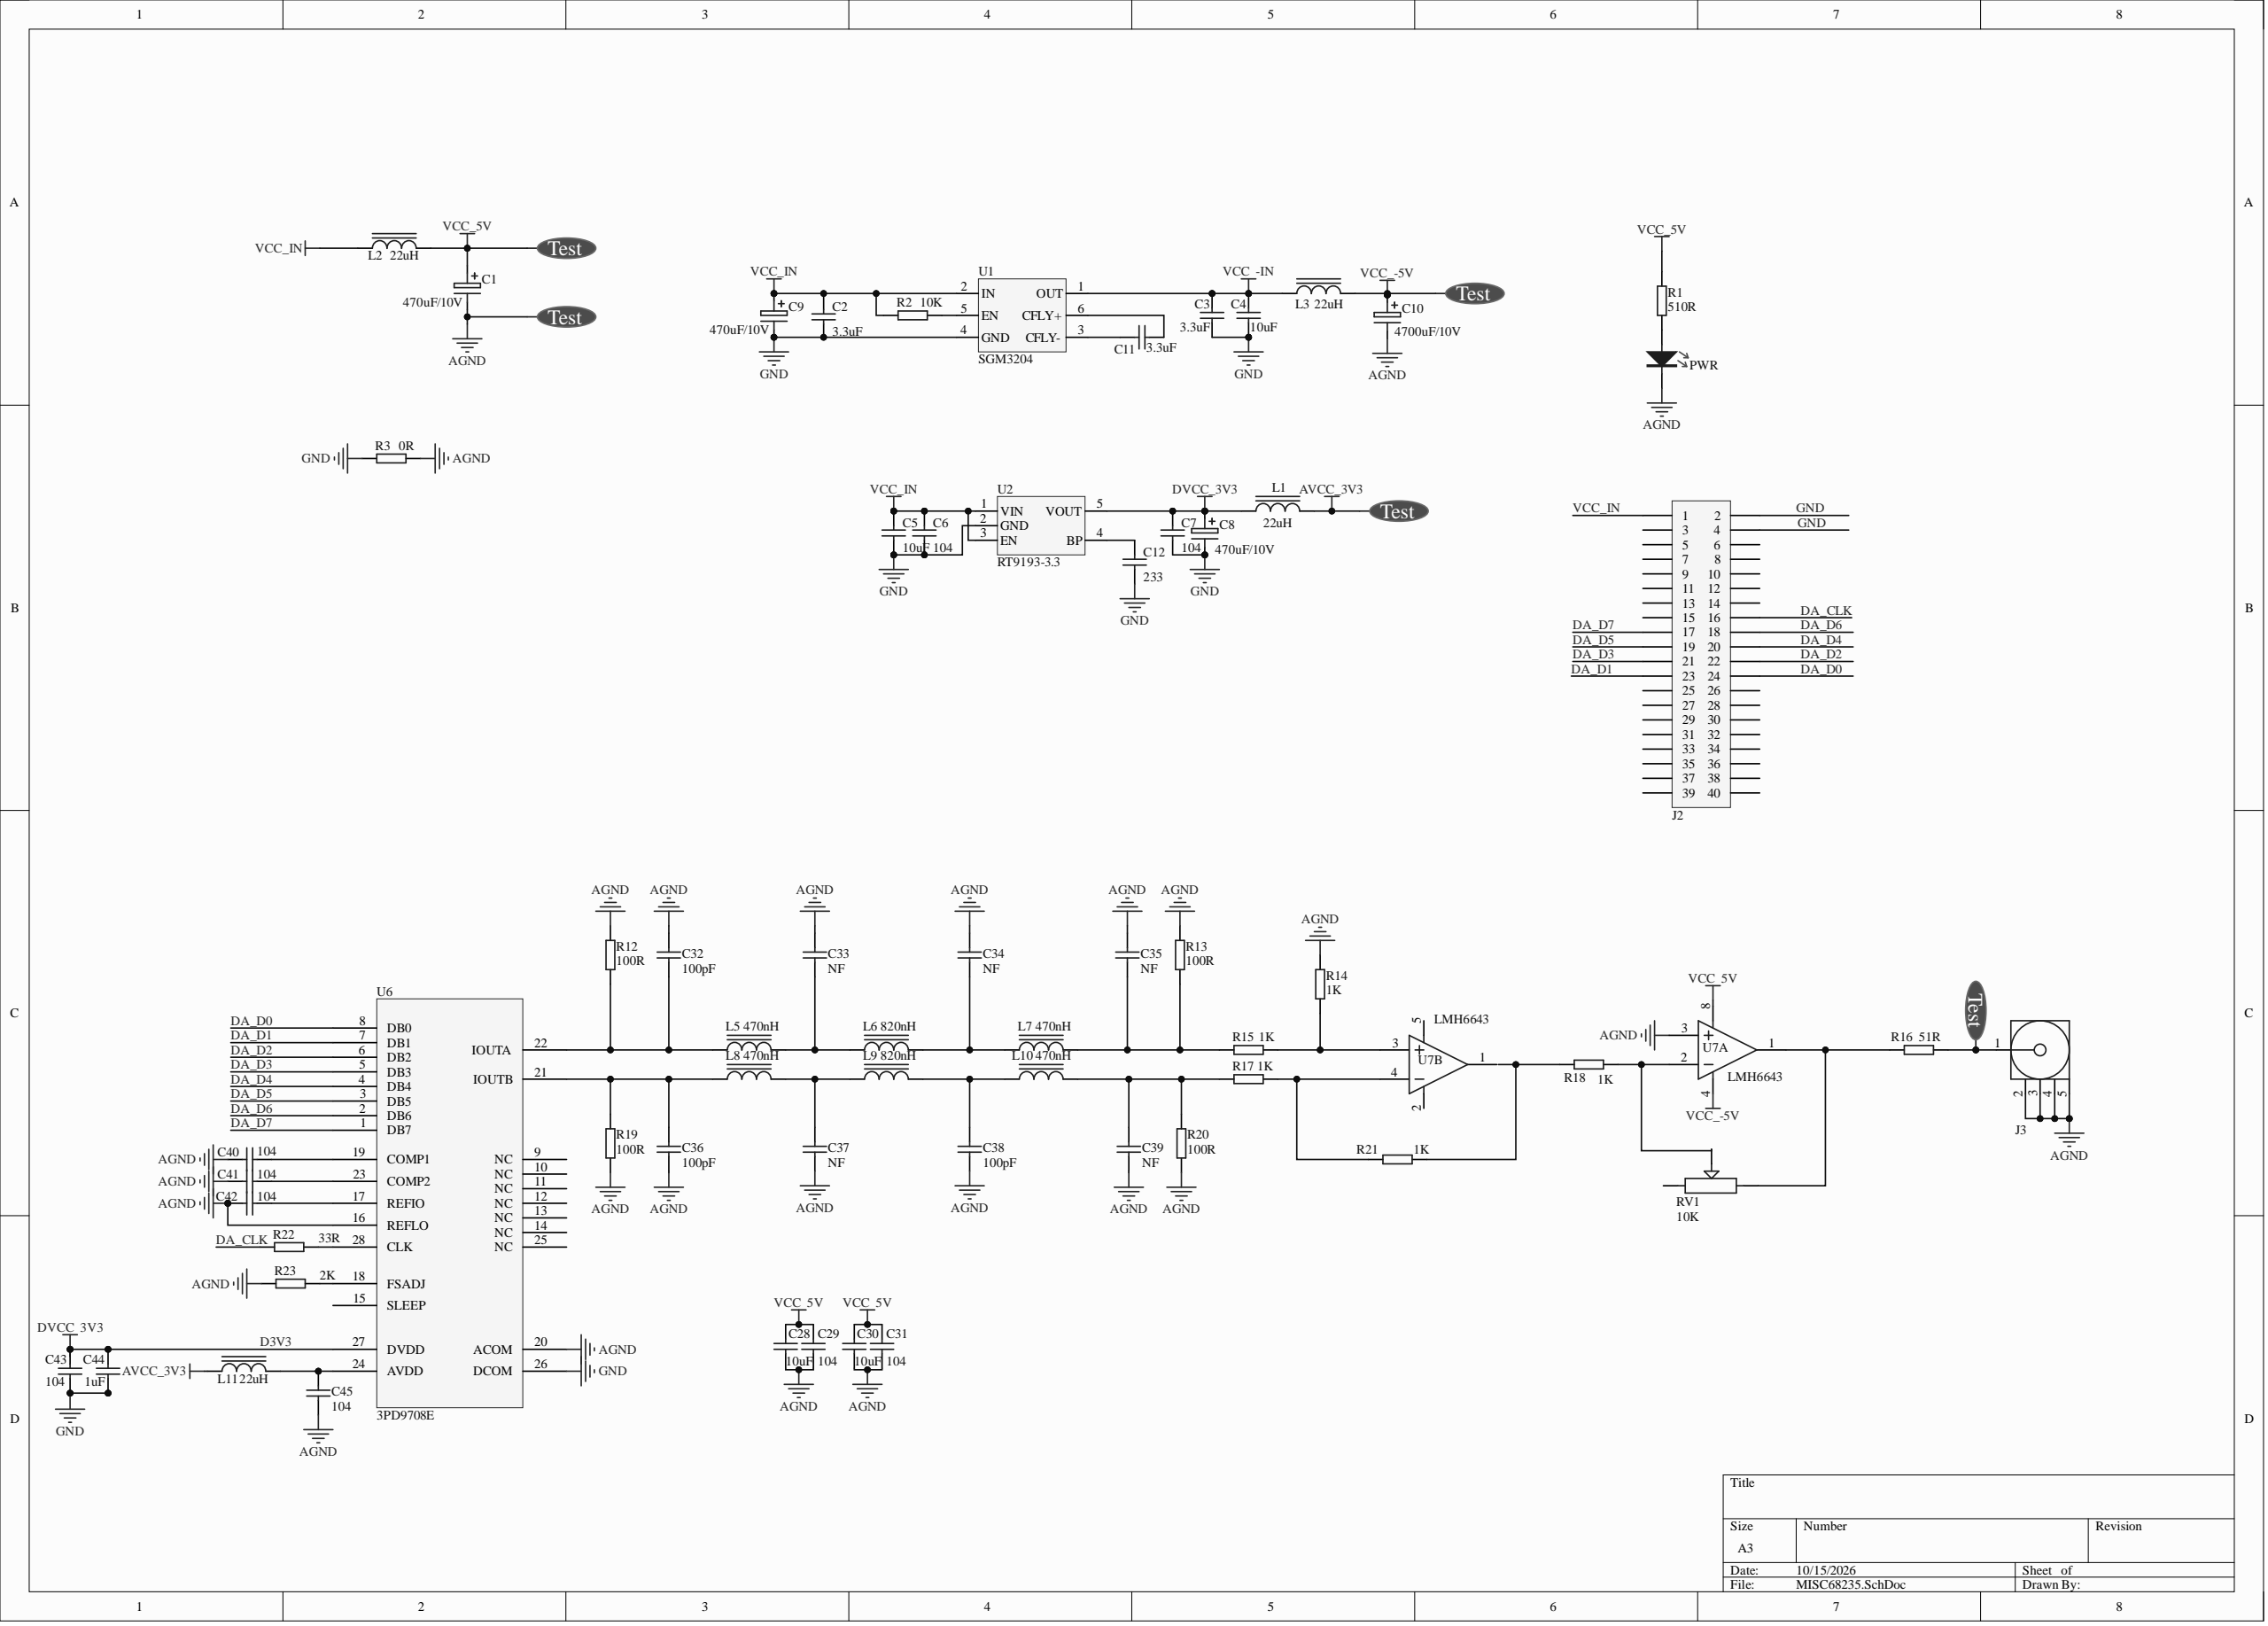Circuit board | Altium Designer | 69 parts | 44 nets
Bill of materials:
Comment,Description,Designator,Footprint,LibRef,Quantity
"470uF/10V","","C1, C8, C9","CS 6.3mm*5.4mm","C-CAP-SMD-220uF/10V","3"
"3.3uF","","C2, C3, C11","CAP-SMD-0603","C-0603-SMD","3"
"10uF","","C4, C5, C28, C30","CAP-SMD-0603","C-0603-SMD","4"
"104","","C6, C7, C29, C31, C40, C41, C42, C43, C45","CAP-SMD-0603","C-0603-SMD","9"
"4700uF/10V","","C10","CS 6.3mm*5.4mm","C-CAP-SMD-220uF/10V","1"
"233","","C12","CAP-SMD-0603","C-0603-SMD","1"
"100pF","","C32, C36, C38","CAP-SMD-0603","C-0603-SMD","3"
"NF","","C33, C34, C35, C37, C39","CAP-SMD-0603","C-0603-SMD","5"
"1uF","","C44","CAP-SMD-0603","C-0603-SMD","1"
"Header-HS_AD_DA-2*20-2.54mm","High-speed AD/DA module interface","J2","HEADER-HS-AD-DA-2*20-2.54MM","Header-HS_AD_DA-2*20-2.54mm","1"
"SMA-KWE","","J3","SMA-KHD","SMA-KWE","1"
"22uH","SMD inductor","L1, L2, L3, L11","RES-SMD-0603","L-0603-SMD","4"
"470nH","SMD inductor","L5, L7, L8, L10","RES-SMD-0603","L-0603-SMD","4"
"820nH","SMD inductor","L6, L9","RES-SMD-0603","L-0603-SMD","2"
"LED-0805","LED","PWR","LED-SMD-0805","LED-0805","1"
"510R","SMD resistor","R1","RES-SMD-0603","R-0603-SMD","1"
"10K","SMD resistor","R2","RES-SMD-0603","R-0603-SMD","1"
"0R","SMD resistor","R3","RES-SMD-0603","R-0603-SMD","1"
"100R","SMD resistor","R12, R13, R19, R20","RES-SMD-0603","R-0603-SMD","4"
"1K","SMD resistor","R14, R15, R17, R18, R21","RES-SMD-0603","R-0603-SMD","5"
"51R","SMD resistor","R16","RES-SMD-0603","R-0603-SMD","1"
"33R","SMD resistor","R22","RES-SMD-0603","R-0603-SMD","1"
"2K","SMD resistor","R23","RES-SMD-0603","R-0603-SMD","1"
"10K","RV09 adjustable potentiometer","RV1","RES-RV09","R-RV09","1"
"Test","Test point","Test1, Test2, Test3, Test4, Test5","Test","Test","5"
"SGM3204","LDO, negative output, 200mA","U1","SOT-23-6","U-SGM3204","1"
"RT9193-3.3","","U2","SOT-23-5","RT9193-3.3","1"
"3PD9708E","High-speed DAC, 8bit/125MSPS","U6","TSSOP-28-NoHot","U-AD9708","1"
"LMH6643","High-speed op amp, 145MHz, 2CH","U7","SOIC-8","U-AD8066","1"
"LMH6643","High-speed op amp, 145MHz, 1CH","U7B","SOT-23-5","U-AD8065","1"
Netlist (Protel format):
[
C1
CS 6.3mm*5.4mm
470uF/10V



]
[
C2
CAP-SMD-0603
3.3uF



]
[
C3
CAP-SMD-0603
3.3uF



]
[
C4
CAP-SMD-0603
10uF



]
[
C5
CAP-SMD-0603
10uF



]
[
C6
CAP-SMD-0603
104



]
[
C7
CAP-SMD-0603
104



]
[
C8
CS 6.3mm*5.4mm
470uF/10V



]
[
C9
CS 6.3mm*5.4mm
470uF/10V



]
[
C10
CS 6.3mm*5.4mm
4700uF/10V



]
[
C11
CAP-SMD-0603
3.3uF



]
[
C12
CAP-SMD-0603
233



]
[
C28
CAP-SMD-0603
10uF



]
[
C29
CAP-SMD-0603
104



]
[
C30
CAP-SMD-0603
10uF



]
[
C31
CAP-SMD-0603
104



]
[
C32
CAP-SMD-0603
100pF



]
[
C33
CAP-SMD-0603
NF



]
[
C34
CAP-SMD-0603
NF



]
[
C35
CAP-SMD-0603
NF



]
[
C36
CAP-SMD-0603
100pF



]
[
C37
CAP-SMD-0603
NF



]
[
C38
CAP-SMD-0603
100pF



]
[
C39
CAP-SMD-0603
NF



]
[
C40
CAP-SMD-0603
104



]
[
C41
CAP-SMD-0603
104



]
[
C42
CAP-SMD-0603
104



]
[
C43
CAP-SMD-0603
104



]
[
C44
CAP-SMD-0603
1uF



]
[
C45
CAP-SMD-0603
104



]
[
J2
HEADER-HS-AD-DA-2*20-2.54MM
Header-HS_AD_DA-2*20-2.54mm



]
[
J3
SMA-KHD
SMA-KWE



]
[
L1
RES-SMD-0603
22uH



]
[
L2
RES-SMD-0603
22uH



]
[
L3
RES-SMD-0603
22uH



]
[
L5
RES-SMD-0603
470nH



]
[
L6
RES-SMD-0603
820nH



]
[
L7
RES-SMD-0603
470nH



]
[
L8
RES-SMD-0603
470nH



]
[
L9
RES-SMD-0603
820nH



]
[
L10
RES-SMD-0603
470nH



]
[
L11
RES-SMD-0603
22uH



]
[
PWR
LED-SMD-0805
LED-0805



]
[
R1
RES-SMD-0603
510R



]
[
R2
RES-SMD-0603
10K



]
[
R3
RES-SMD-0603
0R



]
[
R12
RES-SMD-0603
100R



]
[
R13
RES-SMD-0603
100R



]
[
R14
RES-SMD-0603
1K



]
[
R15
RES-SMD-0603
1K



]
[
R16
RES-SMD-0603
51R



]
[
R17
RES-SMD-0603
1K



]
[
R18
RES-SMD-0603
1K



]
[
R19
RES-SMD-0603
100R



]
[
R20
RES-SMD-0603
100R



]
[
R21
RES-SMD-0603
1K



]
[
R22
RES-SMD-0603
33R



]
[
R23
RES-SMD-0603
2K



]
[
RV1
RES-RV09
10K



]
[
Test1
Test
Test



]
[
Test2
Test
Test



]
[
Test3
Test
Test



]
[
Test4
Test
Test



]
[
Test5
Test
Test



]
[
U1
SOT-23-6
SGM3204



]
[
U2
SOT-23-5
RT9193-3.3



]
[
U6
TSSOP-28-NoHot
3PD9708E



]
[
U7
SOIC-8
LMH6643



]
[
U7B
SOT-23-5
LMH6643



]
(
VCC_IN
C2-2
C5-2
C6-2
C9-1
J2-1
L2-2
R2-1
U1-2
U2-1
U2-3
)
(
VCC_-5V
C10-1
L3-1
Test3-1
U7-4
)
(
VCC_5V
C1-1
L2-1
R1-1
Test2-1
)
(
VCC  -IN
C3-1
C4-1
L3-2
U1-1
)
(
VCC  5V
C28-2
C29-2
C30-2
C31-2
U7-8
)
(
NetR23_2
R23-2
U6-18
)
(
NetR22_2
R22-2
U6-28
)
(
NetR18_2
R18-2
RV1-2
U7-2
)
(
NetR18_1
R18-1
R21-2
)
(
NetR17_2
R17-2
R21-1
U7B-4
)
(
NetR16_1
R16-1
RV1-3
U7-1
)
(
NetR14_1
R14-1
R15-2
U7B-3
)
(
NetR2_2
R2-2
U1-5
)
(
NetPWR_1
PWR-1
R1-2
)
(
NetJ3_1
J3-1
R16-2
Test1-1
)
(
NetC45_1
C45-1
L11-1
U6-24
)
(
NetC42_1
C42-1
U6-17
)
(
NetC41_1
C41-1
U6-23
)
(
NetC40_2
C40-2
U6-19
)
(
NetC39_2
C39-2
L10-1
R17-1
R20-1
)
(
NetC38_2
C38-2
L9-1
L10-2
)
(
NetC37_2
C37-2
L8-1
L9-2
)
(
NetC36_2
C36-2
L8-2
R19-1
U6-21
)
(
NetC35_2
C35-2
L7-1
R13-1
R15-1
)
(
NetC34_2
C34-2
L6-1
L7-2
)
(
NetC33_2
C33-2
L5-1
L6-2
)
(
NetC32_2
C32-2
L5-2
R12-1
U6-22
)
(
NetC12_2
C12-2
U2-4
)
(
NetC11_2
C11-2
U1-3
)
(
NetC11_1
C11-1
U1-6
)
(
GND
C2-1
C3-2
C4-2
C5-1
C6-1
C7-1
C8-2
C9-2
C12-1
C43-1
C44-1
J2-2
J2-4
R3-1
U1-4
U2-2
U6-26
)
(
DVCC_3V3
C7-2
C8-1
L1-2
U2-5
)
(
DA_D7
J2-17
U6-1
)
(
DA_D6
J2-18
U6-2
)
(
DA_D5
J2-19
U6-3
)
(
DA_D4
J2-20
U6-4
)
(
DA_D3
J2-21
U6-5
)
(
DA_D2
J2-22
U6-6
)
(
DA_D1
J2-23
U6-7
)
(
DA_D0
J2-24
U6-8
)
(
DA_CLK
J2-16
R22-1
)
(
D3V3
C43-2
C44-2
U6-27
)
(
AVCC_3V3
L1-1
L11-2
Test5-1
)
(
AGND
C1-2
C10-2
C28-1
C29-1
C30-1
C31-1
C32-1
C33-1
C34-1
C35-1
C36-1
C37-1
C38-1
C39-1
C40-1
C41-2
C42-2
C45-2
J3-2
J3-3
J3-4
J3-5
PWR-2
R3-2
R12-2
R13-2
R14-2
R19-2
R20-2
R23-1
Test4-1
U6-16
U6-20
U7-3
)